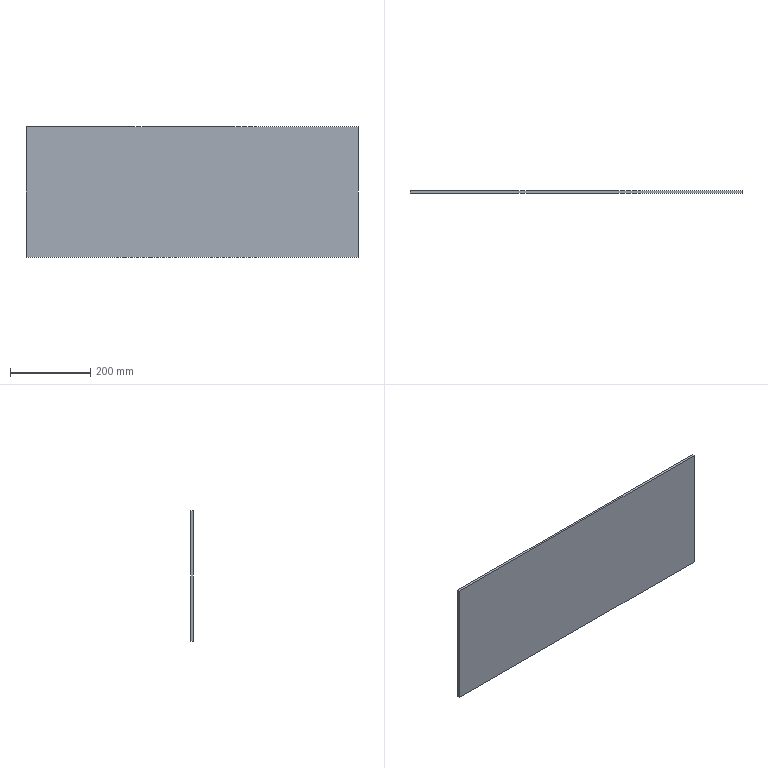Part | STEP file | JBJ-P-1006-12 | 1 solid | 6 faces | box 828 x 6 x 325 mm | volume 1614600 mm3 | plane 6
STEP:
#1=CARTESIAN_POINT('',(414.,0.,162.5));
#2=VERTEX_POINT('',#1);
#3=CARTESIAN_POINT('',(414.,0.,-162.5));
#4=VERTEX_POINT('',#3);
#5=CARTESIAN_POINT('',(414.,0.,-162.5));
#6=DIRECTION('',(0.,0.,-1.));
#7=VECTOR('',#6,1000.);
#8=LINE('',#5,#7);
#9=EDGE_CURVE('',#2,#4,#8,.T.);
#10=ORIENTED_EDGE('',*,*,#9,.T.);
#11=CARTESIAN_POINT('',(414.,6.,-162.5));
#12=VERTEX_POINT('',#11);
#13=CARTESIAN_POINT('',(414.,6.,-162.5));
#14=DIRECTION('',(0.,-1.,0.));
#15=VECTOR('',#14,1000.);
#16=LINE('',#13,#15);
#17=EDGE_CURVE('',#12,#4,#16,.T.);
#18=ORIENTED_EDGE('',*,*,#17,.F.);
#19=CARTESIAN_POINT('',(414.,6.,162.5));
#20=VERTEX_POINT('',#19);
#21=CARTESIAN_POINT('',(414.,6.,-162.5));
#22=DIRECTION('',(0.,0.,-1.));
#23=VECTOR('',#22,1000.);
#24=LINE('',#21,#23);
#25=EDGE_CURVE('',#20,#12,#24,.T.);
#26=ORIENTED_EDGE('',*,*,#25,.F.);
#27=CARTESIAN_POINT('',(414.,6.,162.5));
#28=DIRECTION('',(0.,-1.,0.));
#29=VECTOR('',#28,1000.);
#30=LINE('',#27,#29);
#31=EDGE_CURVE('',#20,#2,#30,.T.);
#32=ORIENTED_EDGE('',*,*,#31,.T.);
#33=EDGE_LOOP('',(#10,#18,#26,#32));
#34=FACE_OUTER_BOUND('',#33,.T.);
#35=CARTESIAN_POINT('',(414.,6.,-162.5));
#36=DIRECTION('',(-1.,0.,0.));
#37=DIRECTION('',(0.,0.,1.));
#38=AXIS2_PLACEMENT_3D('',#35,#36,#37);
#39=PLANE('',#38);
#40=ADVANCED_FACE('',(#34),#39,.F.);
#41=CARTESIAN_POINT('',(-414.,0.,-162.5));
#42=VERTEX_POINT('',#41);
#43=CARTESIAN_POINT('',(-414.,0.,-162.5));
#44=DIRECTION('',(-1.,0.,0.));
#45=VECTOR('',#44,1000.);
#46=LINE('',#43,#45);
#47=EDGE_CURVE('',#4,#42,#46,.T.);
#48=ORIENTED_EDGE('',*,*,#47,.T.);
#49=CARTESIAN_POINT('',(-414.,6.,-162.5));
#50=VERTEX_POINT('',#49);
#51=CARTESIAN_POINT('',(-414.,6.,-162.5));
#52=DIRECTION('',(0.,-1.,0.));
#53=VECTOR('',#52,1000.);
#54=LINE('',#51,#53);
#55=EDGE_CURVE('',#50,#42,#54,.T.);
#56=ORIENTED_EDGE('',*,*,#55,.F.);
#57=CARTESIAN_POINT('',(-414.,6.,-162.5));
#58=DIRECTION('',(-1.,0.,0.));
#59=VECTOR('',#58,1000.);
#60=LINE('',#57,#59);
#61=EDGE_CURVE('',#12,#50,#60,.T.);
#62=ORIENTED_EDGE('',*,*,#61,.F.);
#63=ORIENTED_EDGE('',*,*,#17,.T.);
#64=EDGE_LOOP('',(#48,#56,#62,#63));
#65=FACE_OUTER_BOUND('',#64,.T.);
#66=CARTESIAN_POINT('',(-414.,6.,-162.5));
#67=DIRECTION('',(0.,0.,1.));
#68=DIRECTION('',(1.,0.,0.));
#69=AXIS2_PLACEMENT_3D('',#66,#67,#68);
#70=PLANE('',#69);
#71=ADVANCED_FACE('',(#65),#70,.F.);
#72=CARTESIAN_POINT('',(-414.,0.,162.5));
#73=VERTEX_POINT('',#72);
#74=CARTESIAN_POINT('',(-414.,0.,-162.5));
#75=DIRECTION('',(0.,0.,1.));
#76=VECTOR('',#75,1000.);
#77=LINE('',#74,#76);
#78=EDGE_CURVE('',#42,#73,#77,.T.);
#79=ORIENTED_EDGE('',*,*,#78,.T.);
#80=CARTESIAN_POINT('',(-414.,6.,162.5));
#81=VERTEX_POINT('',#80);
#82=CARTESIAN_POINT('',(-414.,6.,162.5));
#83=DIRECTION('',(0.,-1.,0.));
#84=VECTOR('',#83,1000.);
#85=LINE('',#82,#84);
#86=EDGE_CURVE('',#81,#73,#85,.T.);
#87=ORIENTED_EDGE('',*,*,#86,.F.);
#88=CARTESIAN_POINT('',(-414.,6.,-162.5));
#89=DIRECTION('',(0.,0.,1.));
#90=VECTOR('',#89,1000.);
#91=LINE('',#88,#90);
#92=EDGE_CURVE('',#50,#81,#91,.T.);
#93=ORIENTED_EDGE('',*,*,#92,.F.);
#94=ORIENTED_EDGE('',*,*,#55,.T.);
#95=EDGE_LOOP('',(#79,#87,#93,#94));
#96=FACE_OUTER_BOUND('',#95,.T.);
#97=CARTESIAN_POINT('',(-414.,6.,-162.5));
#98=DIRECTION('',(1.,0.,0.));
#99=DIRECTION('',(0.,0.,-1.));
#100=AXIS2_PLACEMENT_3D('',#97,#98,#99);
#101=PLANE('',#100);
#102=ADVANCED_FACE('',(#96),#101,.F.);
#103=CARTESIAN_POINT('',(-414.,0.,162.5));
#104=DIRECTION('',(1.,0.,0.));
#105=VECTOR('',#104,1000.);
#106=LINE('',#103,#105);
#107=EDGE_CURVE('',#73,#2,#106,.T.);
#108=ORIENTED_EDGE('',*,*,#107,.T.);
#109=ORIENTED_EDGE('',*,*,#31,.F.);
#110=CARTESIAN_POINT('',(-414.,6.,162.5));
#111=DIRECTION('',(1.,0.,0.));
#112=VECTOR('',#111,1000.);
#113=LINE('',#110,#112);
#114=EDGE_CURVE('',#81,#20,#113,.T.);
#115=ORIENTED_EDGE('',*,*,#114,.F.);
#116=ORIENTED_EDGE('',*,*,#86,.T.);
#117=EDGE_LOOP('',(#108,#109,#115,#116));
#118=FACE_OUTER_BOUND('',#117,.T.);
#119=CARTESIAN_POINT('',(-414.,6.,162.5));
#120=DIRECTION('',(0.,0.,-1.));
#121=DIRECTION('',(-1.,0.,0.));
#122=AXIS2_PLACEMENT_3D('',#119,#120,#121);
#123=PLANE('',#122);
#124=ADVANCED_FACE('',(#118),#123,.F.);
#125=ORIENTED_EDGE('',*,*,#25,.T.);
#126=ORIENTED_EDGE('',*,*,#61,.T.);
#127=ORIENTED_EDGE('',*,*,#92,.T.);
#128=ORIENTED_EDGE('',*,*,#114,.T.);
#129=EDGE_LOOP('',(#125,#126,#127,#128));
#130=FACE_OUTER_BOUND('',#129,.T.);
#131=CARTESIAN_POINT('',(0.,6.,0.));
#132=DIRECTION('',(0.,1.,0.));
#133=DIRECTION('',(0.,0.,1.));
#134=AXIS2_PLACEMENT_3D('',#131,#132,#133);
#135=PLANE('',#134);
#136=ADVANCED_FACE('',(#130),#135,.T.);
#137=ORIENTED_EDGE('',*,*,#9,.F.);
#138=ORIENTED_EDGE('',*,*,#107,.F.);
#139=ORIENTED_EDGE('',*,*,#78,.F.);
#140=ORIENTED_EDGE('',*,*,#47,.F.);
#141=EDGE_LOOP('',(#137,#138,#139,#140));
#142=FACE_OUTER_BOUND('',#141,.T.);
#143=CARTESIAN_POINT('',(0.,0.,0.));
#144=DIRECTION('',(0.,1.,0.));
#145=DIRECTION('',(0.,0.,1.));
#146=AXIS2_PLACEMENT_3D('',#143,#144,#145);
#147=PLANE('',#146);
#148=ADVANCED_FACE('',(#142),#147,.F.);
#149=CLOSED_SHELL('',(#40,#71,#102,#124,#136,#148));
#150=MANIFOLD_SOLID_BREP('',#149);
#151=CARTESIAN_POINT('',(0.,0.,0.));
#152=DIRECTION('',(0.,0.,1.));
#153=DIRECTION('',(1.,0.,0.));
#154=AXIS2_PLACEMENT_3D('',#151,#152,#153);
#155=(LENGTH_UNIT()NAMED_UNIT(*)SI_UNIT(.MILLI.,.METRE.));
#156=UNCERTAINTY_MEASURE_WITH_UNIT(LENGTH_MEASURE(0.00001),#155,'','');
#157=(NAMED_UNIT(*)PLANE_ANGLE_UNIT()SI_UNIT($,.RADIAN.));
#158=(NAMED_UNIT(*)SI_UNIT($,.STERADIAN.)SOLID_ANGLE_UNIT());
#159=(GEOMETRIC_REPRESENTATION_CONTEXT(3)GLOBAL_UNCERTAINTY_ASSIGNED_CONTEXT((#156))GLOBAL_UNIT_ASSIGNED_CONTEXT((#155,#157,#158))REPRESENTATION_CONTEXT('',''));
#160=ADVANCED_BREP_SHAPE_REPRESENTATION('',(#150,#154),#159);